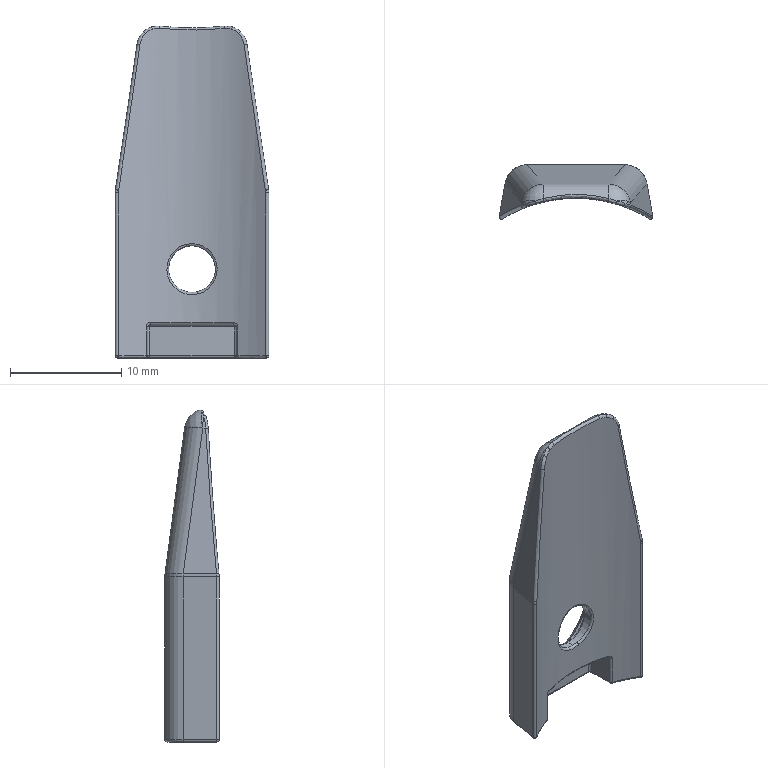Part | STEP file | 101000007696 | 1 solid | 92 faces | box 13.848 x 4.891 x 29.9 mm | volume 904.543 mm3 | cylinder 32 | spline 19 | sphere 15 | plane 13 | torus 9 | cone 4 | commonest cylinder face diameters 0.4 x17 4 x10 4.2 x2 8 x2 25.4 x1